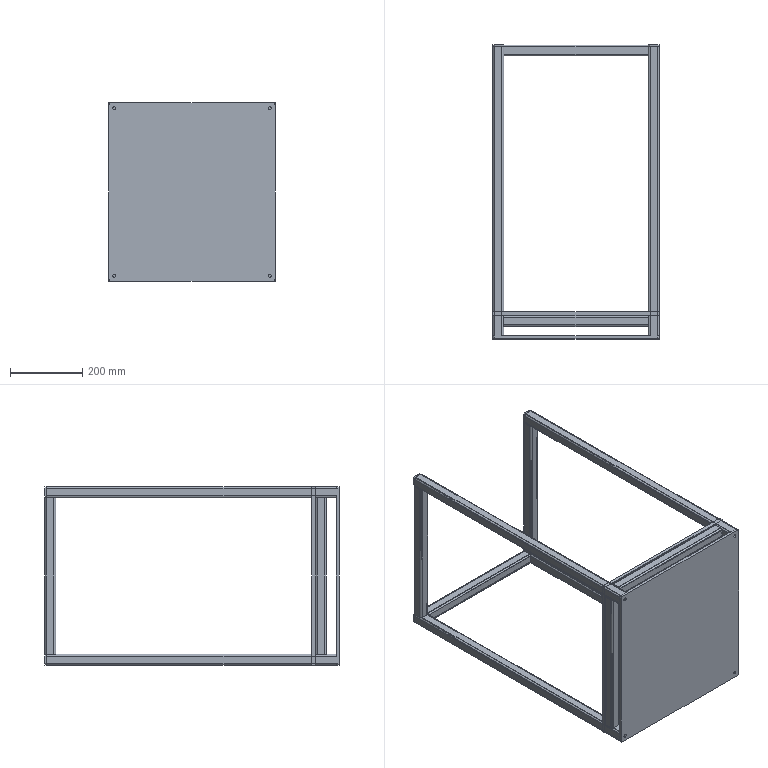Part | STEP file | Lift frame (default_machined_) | 13 solids | 254 faces | box 460 x 814 x 493 mm | volume 5738734 mm3 | plane 154 | cylinder 100 | commonest cylinder face diameters 10.4 x48 5.2 x44 8.5 x8